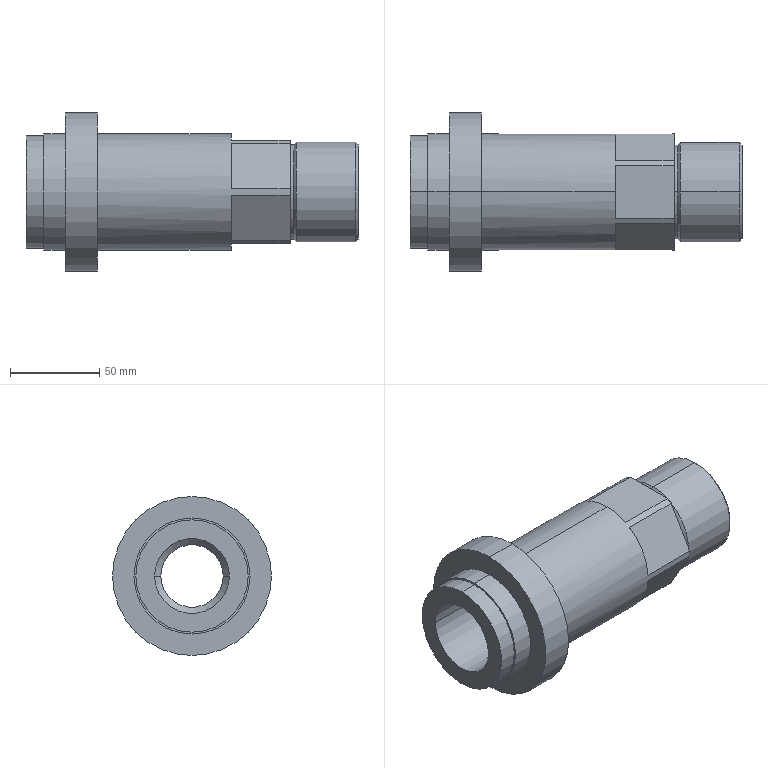Part | SolidWorks | features Chamfer 2, CirPattern 1, ICE 1, RevCut 1, Revolution 1 | 1 solid | 42 faces | box 186 x 89 x 89 mm | volume 390836 mm3 | plane 18 | cylinder 16 | cone 8 | commonest cylinder face diameters 65 x4 35 x2 42 x2 53 x2 56 x2 63 x2
STEP:
#1=CARTESIAN_POINT('',(-3.5,-17.5,0.));
#2=VERTEX_POINT('',#1);
#3=CARTESIAN_POINT('',(-3.5,17.5,0.));
#4=VERTEX_POINT('',#3);
#5=CARTESIAN_POINT('',(-3.5,0.,0.));
#6=DIRECTION('',(1.,0.,0.));
#7=DIRECTION('',(0.,1.,0.));
#8=AXIS2_PLACEMENT_3D('',#5,#6,#7);
#9=CIRCLE('',#8,17.5);
#10=EDGE_CURVE('',#2,#4,#9,.T.);
#11=ORIENTED_EDGE('',*,*,#10,.F.);
#12=CARTESIAN_POINT('',(0.,-21.,0.));
#13=VERTEX_POINT('',#12);
#14=CARTESIAN_POINT('',(-3.5,-17.5,0.));
#15=DIRECTION('',(0.7071,-0.7071,0.));
#16=VECTOR('',#15,1000.);
#17=LINE('',#14,#16);
#18=EDGE_CURVE('',#2,#13,#17,.T.);
#19=ORIENTED_EDGE('',*,*,#18,.T.);
#20=CARTESIAN_POINT('',(0.,21.,0.));
#21=VERTEX_POINT('',#20);
#22=CARTESIAN_POINT('',(0.,0.,0.));
#23=DIRECTION('',(-1.,0.,0.));
#24=DIRECTION('',(0.,0.,-1.));
#25=AXIS2_PLACEMENT_3D('',#22,#23,#24);
#26=CIRCLE('',#25,21.);
#27=EDGE_CURVE('',#21,#13,#26,.T.);
#28=ORIENTED_EDGE('',*,*,#27,.F.);
#29=CARTESIAN_POINT('',(-3.5,17.5,0.));
#30=DIRECTION('',(0.7071,0.7071,0.));
#31=VECTOR('',#30,1000.);
#32=LINE('',#29,#31);
#33=EDGE_CURVE('',#4,#21,#32,.T.);
#34=ORIENTED_EDGE('',*,*,#33,.F.);
#35=EDGE_LOOP('',(#11,#19,#28,#34));
#36=FACE_OUTER_BOUND('',#35,.T.);
#37=CARTESIAN_POINT('',(-3.5,0.,0.));
#38=DIRECTION('',(1.,0.,0.));
#39=DIRECTION('',(0.,1.,0.));
#40=AXIS2_PLACEMENT_3D('',#37,#38,#39);
#41=CONICAL_SURFACE('',#40,17.5,0.7854);
#42=ADVANCED_FACE('',(#36),#41,.F.);
#43=CARTESIAN_POINT('',(-186.,-21.,0.));
#44=VERTEX_POINT('',#43);
#45=CARTESIAN_POINT('',(-186.,21.,0.));
#46=VERTEX_POINT('',#45);
#47=CARTESIAN_POINT('',(-186.,0.,0.));
#48=DIRECTION('',(1.,0.,0.));
#49=DIRECTION('',(0.,1.,0.));
#50=AXIS2_PLACEMENT_3D('',#47,#48,#49);
#51=CIRCLE('',#50,21.);
#52=EDGE_CURVE('',#44,#46,#51,.T.);
#53=ORIENTED_EDGE('',*,*,#52,.F.);
#54=CARTESIAN_POINT('',(-70.,-21.,0.));
#55=VERTEX_POINT('',#54);
#56=CARTESIAN_POINT('',(0.,-21.,0.));
#57=DIRECTION('',(1.,0.,0.));
#58=VECTOR('',#57,1000.);
#59=LINE('',#56,#58);
#60=EDGE_CURVE('',#44,#55,#59,.T.);
#61=ORIENTED_EDGE('',*,*,#60,.T.);
#62=CARTESIAN_POINT('',(-70.,21.,0.));
#63=VERTEX_POINT('',#62);
#64=CARTESIAN_POINT('',(-70.,0.,0.));
#65=DIRECTION('',(1.,0.,0.));
#66=DIRECTION('',(0.,1.,0.));
#67=AXIS2_PLACEMENT_3D('',#64,#65,#66);
#68=CIRCLE('',#67,21.);
#69=EDGE_CURVE('',#55,#63,#68,.T.);
#70=ORIENTED_EDGE('',*,*,#69,.T.);
#71=CARTESIAN_POINT('',(0.,21.,0.));
#72=DIRECTION('',(1.,0.,0.));
#73=VECTOR('',#72,1000.);
#74=LINE('',#71,#73);
#75=EDGE_CURVE('',#46,#63,#74,.T.);
#76=ORIENTED_EDGE('',*,*,#75,.F.);
#77=EDGE_LOOP('',(#53,#61,#70,#76));
#78=FACE_OUTER_BOUND('',#77,.T.);
#79=CARTESIAN_POINT('',(0.,0.,0.));
#80=DIRECTION('',(1.,0.,0.));
#81=DIRECTION('',(0.,1.,0.));
#82=AXIS2_PLACEMENT_3D('',#79,#80,#81);
#83=CYLINDRICAL_SURFACE('',#82,21.);
#84=ADVANCED_FACE('',(#78),#83,.F.);
#85=CARTESIAN_POINT('',(-66.5,-17.5,0.));
#86=VERTEX_POINT('',#85);
#87=CARTESIAN_POINT('',(-66.5,17.5,0.));
#88=VERTEX_POINT('',#87);
#89=CARTESIAN_POINT('',(-66.5,0.,0.));
#90=DIRECTION('',(1.,0.,0.));
#91=DIRECTION('',(0.,1.,0.));
#92=AXIS2_PLACEMENT_3D('',#89,#90,#91);
#93=CIRCLE('',#92,17.5);
#94=EDGE_CURVE('',#86,#88,#93,.T.);
#95=ORIENTED_EDGE('',*,*,#94,.T.);
#96=CARTESIAN_POINT('',(-66.5,17.5,0.));
#97=DIRECTION('',(-0.7071,0.7071,0.));
#98=VECTOR('',#97,1000.);
#99=LINE('',#96,#98);
#100=EDGE_CURVE('',#88,#63,#99,.T.);
#101=ORIENTED_EDGE('',*,*,#100,.T.);
#102=ORIENTED_EDGE('',*,*,#69,.F.);
#103=CARTESIAN_POINT('',(-66.5,-17.5,0.));
#104=DIRECTION('',(-0.7071,-0.7071,0.));
#105=VECTOR('',#104,1000.);
#106=LINE('',#103,#105);
#107=EDGE_CURVE('',#86,#55,#106,.T.);
#108=ORIENTED_EDGE('',*,*,#107,.F.);
#109=EDGE_LOOP('',(#95,#101,#102,#108));
#110=FACE_OUTER_BOUND('',#109,.T.);
#111=CARTESIAN_POINT('',(-66.5,0.,0.));
#112=DIRECTION('',(-1.,0.,0.));
#113=DIRECTION('',(0.,-1.,0.));
#114=AXIS2_PLACEMENT_3D('',#111,#112,#113);
#115=CONICAL_SURFACE('',#114,17.5,0.7854);
#116=ADVANCED_FACE('',(#110),#115,.F.);
#117=ORIENTED_EDGE('',*,*,#94,.F.);
#118=CARTESIAN_POINT('',(0.,-17.5,0.));
#119=DIRECTION('',(1.,0.,0.));
#120=VECTOR('',#119,1000.);
#121=LINE('',#118,#120);
#122=EDGE_CURVE('',#86,#2,#121,.T.);
#123=ORIENTED_EDGE('',*,*,#122,.T.);
#124=ORIENTED_EDGE('',*,*,#10,.T.);
#125=CARTESIAN_POINT('',(0.,17.5,0.));
#126=DIRECTION('',(1.,0.,0.));
#127=VECTOR('',#126,1000.);
#128=LINE('',#125,#127);
#129=EDGE_CURVE('',#88,#4,#128,.T.);
#130=ORIENTED_EDGE('',*,*,#129,.F.);
#131=EDGE_LOOP('',(#117,#123,#124,#130));
#132=FACE_OUTER_BOUND('',#131,.T.);
#133=CARTESIAN_POINT('',(0.,0.,0.));
#134=DIRECTION('',(1.,0.,0.));
#135=DIRECTION('',(0.,1.,0.));
#136=AXIS2_PLACEMENT_3D('',#133,#134,#135);
#137=CYLINDRICAL_SURFACE('',#136,17.5);
#138=ADVANCED_FACE('',(#132),#137,.F.);
#139=CARTESIAN_POINT('',(0.,0.,-26.5));
#140=VERTEX_POINT('',#139);
#141=CARTESIAN_POINT('',(0.,0.,26.5));
#142=VERTEX_POINT('',#141);
#143=CARTESIAN_POINT('',(0.,0.,0.));
#144=DIRECTION('',(1.,0.,0.));
#145=DIRECTION('',(0.,0.,-1.));
#146=AXIS2_PLACEMENT_3D('',#143,#144,#145);
#147=CIRCLE('',#146,26.5);
#148=EDGE_CURVE('',#140,#142,#147,.T.);
#149=ORIENTED_EDGE('',*,*,#148,.F.);
#150=CARTESIAN_POINT('',(-1.5,0.,-28.));
#151=VERTEX_POINT('',#150);
#152=CARTESIAN_POINT('',(0.,0.,-26.5));
#153=DIRECTION('',(-0.7071,0.,-0.7071));
#154=VECTOR('',#153,1000.);
#155=LINE('',#152,#154);
#156=EDGE_CURVE('',#140,#151,#155,.T.);
#157=ORIENTED_EDGE('',*,*,#156,.T.);
#158=CARTESIAN_POINT('',(-1.5,0.,28.));
#159=VERTEX_POINT('',#158);
#160=CARTESIAN_POINT('',(-1.5,0.,0.));
#161=DIRECTION('',(-1.,0.,0.));
#162=DIRECTION('',(0.,0.,-1.));
#163=AXIS2_PLACEMENT_3D('',#160,#161,#162);
#164=CIRCLE('',#163,28.);
#165=EDGE_CURVE('',#159,#151,#164,.T.);
#166=ORIENTED_EDGE('',*,*,#165,.F.);
#167=CARTESIAN_POINT('',(0.,0.,26.5));
#168=DIRECTION('',(-0.7071,0.,0.7071));
#169=VECTOR('',#168,1000.);
#170=LINE('',#167,#169);
#171=EDGE_CURVE('',#142,#159,#170,.T.);
#172=ORIENTED_EDGE('',*,*,#171,.F.);
#173=EDGE_LOOP('',(#149,#157,#166,#172));
#174=FACE_OUTER_BOUND('',#173,.T.);
#175=CARTESIAN_POINT('',(0.,0.,0.));
#176=DIRECTION('',(-1.,0.,0.));
#177=DIRECTION('',(0.,0.,1.));
#178=AXIS2_PLACEMENT_3D('',#175,#176,#177);
#179=CONICAL_SURFACE('',#178,26.5,0.7854);
#180=ADVANCED_FACE('',(#174),#179,.T.);
#181=CARTESIAN_POINT('',(-36.,0.,-26.5));
#182=VERTEX_POINT('',#181);
#183=CARTESIAN_POINT('',(-36.,0.,26.5));
#184=VERTEX_POINT('',#183);
#185=CARTESIAN_POINT('',(-36.,0.,0.));
#186=DIRECTION('',(1.,0.,0.));
#187=DIRECTION('',(0.,0.,-1.));
#188=AXIS2_PLACEMENT_3D('',#185,#186,#187);
#189=CIRCLE('',#188,26.5);
#190=EDGE_CURVE('',#182,#184,#189,.T.);
#191=ORIENTED_EDGE('',*,*,#190,.T.);
#192=CARTESIAN_POINT('',(-34.5,0.,28.));
#193=VERTEX_POINT('',#192);
#194=CARTESIAN_POINT('',(-36.,0.,26.5));
#195=DIRECTION('',(0.7071,0.,0.7071));
#196=VECTOR('',#195,1000.);
#197=LINE('',#194,#196);
#198=EDGE_CURVE('',#184,#193,#197,.T.);
#199=ORIENTED_EDGE('',*,*,#198,.T.);
#200=CARTESIAN_POINT('',(-34.5,0.,-28.));
#201=VERTEX_POINT('',#200);
#202=CARTESIAN_POINT('',(-34.5,0.,0.));
#203=DIRECTION('',(1.,0.,0.));
#204=DIRECTION('',(0.,0.,-1.));
#205=AXIS2_PLACEMENT_3D('',#202,#203,#204);
#206=CIRCLE('',#205,28.);
#207=EDGE_CURVE('',#201,#193,#206,.T.);
#208=ORIENTED_EDGE('',*,*,#207,.F.);
#209=CARTESIAN_POINT('',(-36.,0.,-26.5));
#210=DIRECTION('',(0.7071,0.,-0.7071));
#211=VECTOR('',#210,1000.);
#212=LINE('',#209,#211);
#213=EDGE_CURVE('',#182,#201,#212,.T.);
#214=ORIENTED_EDGE('',*,*,#213,.F.);
#215=EDGE_LOOP('',(#191,#199,#208,#214));
#216=FACE_OUTER_BOUND('',#215,.T.);
#217=CARTESIAN_POINT('',(-36.,0.,0.));
#218=DIRECTION('',(1.,0.,0.));
#219=DIRECTION('',(0.,0.,-1.));
#220=AXIS2_PLACEMENT_3D('',#217,#218,#219);
#221=CONICAL_SURFACE('',#220,26.5,0.7854);
#222=ADVANCED_FACE('',(#216),#221,.T.);
#223=ORIENTED_EDGE('',*,*,#207,.T.);
#224=CARTESIAN_POINT('',(0.,0.,28.));
#225=DIRECTION('',(1.,0.,0.));
#226=VECTOR('',#225,1000.);
#227=LINE('',#224,#226);
#228=EDGE_CURVE('',#193,#159,#227,.T.);
#229=ORIENTED_EDGE('',*,*,#228,.T.);
#230=ORIENTED_EDGE('',*,*,#165,.T.);
#231=CARTESIAN_POINT('',(0.,0.,-28.));
#232=DIRECTION('',(1.,0.,0.));
#233=VECTOR('',#232,1000.);
#234=LINE('',#231,#233);
#235=EDGE_CURVE('',#201,#151,#234,.T.);
#236=ORIENTED_EDGE('',*,*,#235,.F.);
#237=EDGE_LOOP('',(#223,#229,#230,#236));
#238=FACE_OUTER_BOUND('',#237,.T.);
#239=CARTESIAN_POINT('',(0.,0.,0.));
#240=DIRECTION('',(1.,0.,0.));
#241=DIRECTION('',(0.,0.,-1.));
#242=AXIS2_PLACEMENT_3D('',#239,#240,#241);
#243=CYLINDRICAL_SURFACE('',#242,28.);
#244=ADVANCED_FACE('',(#238),#243,.T.);
#245=CARTESIAN_POINT('',(-186.,0.,-31.5));
#246=VERTEX_POINT('',#245);
#247=CARTESIAN_POINT('',(-186.,0.,31.5));
#248=VERTEX_POINT('',#247);
#249=CARTESIAN_POINT('',(-186.,0.,0.));
#250=DIRECTION('',(1.,0.,0.));
#251=DIRECTION('',(0.,0.,-1.));
#252=AXIS2_PLACEMENT_3D('',#249,#250,#251);
#253=CIRCLE('',#252,31.5);
#254=EDGE_CURVE('',#246,#248,#253,.T.);
#255=ORIENTED_EDGE('',*,*,#254,.T.);
#256=CARTESIAN_POINT('',(-176.,0.,31.5));
#257=VERTEX_POINT('',#256);
#258=CARTESIAN_POINT('',(0.,0.,31.5));
#259=DIRECTION('',(1.,0.,0.));
#260=VECTOR('',#259,1000.);
#261=LINE('',#258,#260);
#262=EDGE_CURVE('',#248,#257,#261,.T.);
#263=ORIENTED_EDGE('',*,*,#262,.T.);
#264=CARTESIAN_POINT('',(-176.,0.,-31.5));
#265=VERTEX_POINT('',#264);
#266=CARTESIAN_POINT('',(-176.,0.,0.));
#267=DIRECTION('',(1.,0.,0.));
#268=DIRECTION('',(0.,0.,-1.));
#269=AXIS2_PLACEMENT_3D('',#266,#267,#268);
#270=CIRCLE('',#269,31.5);
#271=EDGE_CURVE('',#265,#257,#270,.T.);
#272=ORIENTED_EDGE('',*,*,#271,.F.);
#273=CARTESIAN_POINT('',(0.,0.,-31.5));
#274=DIRECTION('',(1.,0.,0.));
#275=VECTOR('',#274,1000.);
#276=LINE('',#273,#275);
#277=EDGE_CURVE('',#246,#265,#276,.T.);
#278=ORIENTED_EDGE('',*,*,#277,.F.);
#279=EDGE_LOOP('',(#255,#263,#272,#278));
#280=FACE_OUTER_BOUND('',#279,.T.);
#281=CARTESIAN_POINT('',(0.,0.,0.));
#282=DIRECTION('',(1.,0.,0.));
#283=DIRECTION('',(0.,0.,-1.));
#284=AXIS2_PLACEMENT_3D('',#281,#282,#283);
#285=CYLINDRICAL_SURFACE('',#284,31.5);
#286=ADVANCED_FACE('',(#280),#285,.T.);
#287=CARTESIAN_POINT('',(-176.,0.,-32.5));
#288=VERTEX_POINT('',#287);
#289=CARTESIAN_POINT('',(-176.,0.,32.5));
#290=VERTEX_POINT('',#289);
#291=CARTESIAN_POINT('',(-176.,0.,0.));
#292=DIRECTION('',(1.,0.,0.));
#293=DIRECTION('',(0.,0.,-1.));
#294=AXIS2_PLACEMENT_3D('',#291,#292,#293);
#295=CIRCLE('',#294,32.5);
#296=EDGE_CURVE('',#288,#290,#295,.T.);
#297=ORIENTED_EDGE('',*,*,#296,.T.);
#298=CARTESIAN_POINT('',(-164.,0.,32.5));
#299=VERTEX_POINT('',#298);
#300=CARTESIAN_POINT('',(0.,0.,32.5));
#301=DIRECTION('',(1.,0.,0.));
#302=VECTOR('',#301,1000.);
#303=LINE('',#300,#302);
#304=EDGE_CURVE('',#290,#299,#303,.T.);
#305=ORIENTED_EDGE('',*,*,#304,.T.);
#306=CARTESIAN_POINT('',(-164.,0.,-32.5));
#307=VERTEX_POINT('',#306);
#308=CARTESIAN_POINT('',(-164.,0.,0.));
#309=DIRECTION('',(1.,0.,0.));
#310=DIRECTION('',(0.,0.,-1.));
#311=AXIS2_PLACEMENT_3D('',#308,#309,#310);
#312=CIRCLE('',#311,32.5);
#313=EDGE_CURVE('',#307,#299,#312,.T.);
#314=ORIENTED_EDGE('',*,*,#313,.F.);
#315=CARTESIAN_POINT('',(0.,0.,-32.5));
#316=DIRECTION('',(1.,0.,0.));
#317=VECTOR('',#316,1000.);
#318=LINE('',#315,#317);
#319=EDGE_CURVE('',#288,#307,#318,.T.);
#320=ORIENTED_EDGE('',*,*,#319,.F.);
#321=EDGE_LOOP('',(#297,#305,#314,#320));
#322=FACE_OUTER_BOUND('',#321,.T.);
#323=CARTESIAN_POINT('',(0.,0.,0.));
#324=DIRECTION('',(1.,0.,0.));
#325=DIRECTION('',(0.,0.,-1.));
#326=AXIS2_PLACEMENT_3D('',#323,#324,#325);
#327=CYLINDRICAL_SURFACE('',#326,32.5);
#328=ADVANCED_FACE('',(#322),#327,.T.);
#329=CARTESIAN_POINT('',(-164.,0.,-44.5));
#330=VERTEX_POINT('',#329);
#331=CARTESIAN_POINT('',(-164.,0.,44.5));
#332=VERTEX_POINT('',#331);
#333=CARTESIAN_POINT('',(-164.,0.,0.));
#334=DIRECTION('',(1.,0.,0.));
#335=DIRECTION('',(0.,0.,-1.));
#336=AXIS2_PLACEMENT_3D('',#333,#334,#335);
#337=CIRCLE('',#336,44.5);
#338=EDGE_CURVE('',#330,#332,#337,.T.);
#339=ORIENTED_EDGE('',*,*,#338,.T.);
#340=CARTESIAN_POINT('',(-146.,0.,44.5));
#341=VERTEX_POINT('',#340);
#342=CARTESIAN_POINT('',(0.,0.,44.5));
#343=DIRECTION('',(1.,0.,0.));
#344=VECTOR('',#343,1000.);
#345=LINE('',#342,#344);
#346=EDGE_CURVE('',#332,#341,#345,.T.);
#347=ORIENTED_EDGE('',*,*,#346,.T.);
#348=CARTESIAN_POINT('',(-146.,0.,-44.5));
#349=VERTEX_POINT('',#348);
#350=CARTESIAN_POINT('',(-146.,0.,0.));
#351=DIRECTION('',(1.,0.,0.));
#352=DIRECTION('',(0.,0.,-1.));
#353=AXIS2_PLACEMENT_3D('',#350,#351,#352);
#354=CIRCLE('',#353,44.5);
#355=EDGE_CURVE('',#349,#341,#354,.T.);
#356=ORIENTED_EDGE('',*,*,#355,.F.);
#357=CARTESIAN_POINT('',(0.,0.,-44.5));
#358=DIRECTION('',(1.,0.,0.));
#359=VECTOR('',#358,1000.);
#360=LINE('',#357,#359);
#361=EDGE_CURVE('',#330,#349,#360,.T.);
#362=ORIENTED_EDGE('',*,*,#361,.F.);
#363=EDGE_LOOP('',(#339,#347,#356,#362));
#364=FACE_OUTER_BOUND('',#363,.T.);
#365=CARTESIAN_POINT('',(0.,0.,0.));
#366=DIRECTION('',(1.,0.,0.));
#367=DIRECTION('',(0.,0.,-1.));
#368=AXIS2_PLACEMENT_3D('',#365,#366,#367);
#369=CYLINDRICAL_SURFACE('',#368,44.5);
#370=ADVANCED_FACE('',(#364),#369,.T.);
#371=CARTESIAN_POINT('',(-146.,0.,-32.5));
#372=VERTEX_POINT('',#371);
#373=CARTESIAN_POINT('',(-146.,0.,32.5));
#374=VERTEX_POINT('',#373);
#375=CARTESIAN_POINT('',(-146.,0.,0.));
#376=DIRECTION('',(1.,0.,0.));
#377=DIRECTION('',(0.,0.,-1.));
#378=AXIS2_PLACEMENT_3D('',#375,#376,#377);
#379=CIRCLE('',#378,32.5);
#380=EDGE_CURVE('',#372,#374,#379,.T.);
#381=ORIENTED_EDGE('',*,*,#380,.T.);
#382=CARTESIAN_POINT('',(-71.,0.,32.5));
#383=VERTEX_POINT('',#382);
#384=CARTESIAN_POINT('',(0.,0.,32.5));
#385=DIRECTION('',(1.,0.,0.));
#386=VECTOR('',#385,1000.);
#387=LINE('',#384,#386);
#388=EDGE_CURVE('',#374,#383,#387,.T.);
#389=ORIENTED_EDGE('',*,*,#388,.T.);
#390=CARTESIAN_POINT('',(-71.,14.671,29.));
#391=VERTEX_POINT('',#390);
#392=CARTESIAN_POINT('',(-71.,0.,0.));
#393=DIRECTION('',(1.,0.,0.));
#394=DIRECTION('',(0.,0.,-1.));
#395=AXIS2_PLACEMENT_3D('',#392,#393,#394);
#396=CIRCLE('',#395,32.5);
#397=EDGE_CURVE('',#391,#383,#396,.T.);
#398=ORIENTED_EDGE('',*,*,#397,.F.);
#399=CARTESIAN_POINT('',(-38.,14.671,29.));
#400=VERTEX_POINT('',#399);
#401=CARTESIAN_POINT('',(-71.,14.671,29.));
#402=DIRECTION('',(1.,0.,0.));
#403=VECTOR('',#402,1000.);
#404=LINE('',#401,#403);
#405=EDGE_CURVE('',#391,#400,#404,.T.);
#406=ORIENTED_EDGE('',*,*,#405,.T.);
#407=CARTESIAN_POINT('',(-38.,17.779,27.206));
#408=VERTEX_POINT('',#407);
#409=CARTESIAN_POINT('',(-38.,0.,0.));
#410=DIRECTION('',(1.,0.,0.));
#411=DIRECTION('',(0.,0.,-1.));
#412=AXIS2_PLACEMENT_3D('',#409,#410,#411);
#413=CIRCLE('',#412,32.5);
#414=EDGE_CURVE('',#408,#400,#413,.T.);
#415=ORIENTED_EDGE('',*,*,#414,.F.);
#416=CARTESIAN_POINT('',(-71.,17.779,27.206));
#417=VERTEX_POINT('',#416);
#418=CARTESIAN_POINT('',(-71.,17.779,27.206));
#419=DIRECTION('',(1.,0.,0.));
#420=VECTOR('',#419,1000.);
#421=LINE('',#418,#420);
#422=EDGE_CURVE('',#417,#408,#421,.T.);
#423=ORIENTED_EDGE('',*,*,#422,.F.);
#424=CARTESIAN_POINT('',(-71.,32.45,1.794));
#425=VERTEX_POINT('',#424);
#426=CARTESIAN_POINT('',(-71.,0.,0.));
#427=DIRECTION('',(1.,0.,0.));
#428=DIRECTION('',(0.,0.,-1.));
#429=AXIS2_PLACEMENT_3D('',#426,#427,#428);
#430=CIRCLE('',#429,32.5);
#431=EDGE_CURVE('',#425,#417,#430,.T.);
#432=ORIENTED_EDGE('',*,*,#431,.F.);
#433=CARTESIAN_POINT('',(-38.,32.45,1.794));
#434=VERTEX_POINT('',#433);
#435=CARTESIAN_POINT('',(-71.,32.45,1.794));
#436=DIRECTION('',(1.,0.,0.));
#437=VECTOR('',#436,1000.);
#438=LINE('',#435,#437);
#439=EDGE_CURVE('',#425,#434,#438,.T.);
#440=ORIENTED_EDGE('',*,*,#439,.T.);
#441=CARTESIAN_POINT('',(-38.,32.45,-1.794));
#442=VERTEX_POINT('',#441);
#443=CARTESIAN_POINT('',(-38.,0.,0.));
#444=DIRECTION('',(1.,0.,0.));
#445=DIRECTION('',(0.,0.,-1.));
#446=AXIS2_PLACEMENT_3D('',#443,#444,#445);
#447=CIRCLE('',#446,32.5);
#448=EDGE_CURVE('',#442,#434,#447,.T.);
#449=ORIENTED_EDGE('',*,*,#448,.F.);
#450=CARTESIAN_POINT('',(-71.,32.45,-1.794));
#451=VERTEX_POINT('',#450);
#452=CARTESIAN_POINT('',(-71.,32.45,-1.794));
#453=DIRECTION('',(1.,0.,0.));
#454=VECTOR('',#453,1000.);
#455=LINE('',#452,#454);
#456=EDGE_CURVE('',#451,#442,#455,.T.);
#457=ORIENTED_EDGE('',*,*,#456,.F.);
#458=CARTESIAN_POINT('',(-71.,17.779,-27.206));
#459=VERTEX_POINT('',#458);
#460=CARTESIAN_POINT('',(-71.,0.,0.));
#461=DIRECTION('',(1.,0.,0.));
#462=DIRECTION('',(0.,0.,-1.));
#463=AXIS2_PLACEMENT_3D('',#460,#461,#462);
#464=CIRCLE('',#463,32.5);
#465=EDGE_CURVE('',#459,#451,#464,.T.);
#466=ORIENTED_EDGE('',*,*,#465,.F.);
#467=CARTESIAN_POINT('',(-38.,17.779,-27.206));
#468=VERTEX_POINT('',#467);
#469=CARTESIAN_POINT('',(-71.,17.779,-27.206));
#470=DIRECTION('',(1.,0.,0.));
#471=VECTOR('',#470,1000.);
#472=LINE('',#469,#471);
#473=EDGE_CURVE('',#459,#468,#472,.T.);
#474=ORIENTED_EDGE('',*,*,#473,.T.);
#475=CARTESIAN_POINT('',(-38.,14.671,-29.));
#476=VERTEX_POINT('',#475);
#477=CARTESIAN_POINT('',(-38.,0.,0.));
#478=DIRECTION('',(1.,0.,0.));
#479=DIRECTION('',(0.,0.,-1.));
#480=AXIS2_PLACEMENT_3D('',#477,#478,#479);
#481=CIRCLE('',#480,32.5);
#482=EDGE_CURVE('',#476,#468,#481,.T.);
#483=ORIENTED_EDGE('',*,*,#482,.F.);
#484=CARTESIAN_POINT('',(-71.,14.671,-29.));
#485=VERTEX_POINT('',#484);
#486=CARTESIAN_POINT('',(-71.,14.671,-29.));
#487=DIRECTION('',(1.,0.,0.));
#488=VECTOR('',#487,1000.);
#489=LINE('',#486,#488);
#490=EDGE_CURVE('',#485,#476,#489,.T.);
#491=ORIENTED_EDGE('',*,*,#490,.F.);
#492=CARTESIAN_POINT('',(-71.,0.,-32.5));
#493=VERTEX_POINT('',#492);
#494=CARTESIAN_POINT('',(-71.,0.,0.));
#495=DIRECTION('',(1.,0.,0.));
#496=DIRECTION('',(0.,0.,-1.));
#497=AXIS2_PLACEMENT_3D('',#494,#495,#496);
#498=CIRCLE('',#497,32.5);
#499=EDGE_CURVE('',#493,#485,#498,.T.);
#500=ORIENTED_EDGE('',*,*,#499,.F.);
#501=CARTESIAN_POINT('',(0.,0.,-32.5));
#502=DIRECTION('',(1.,0.,0.));
#503=VECTOR('',#502,1000.);
#504=LINE('',#501,#503);
#505=EDGE_CURVE('',#372,#493,#504,.T.);
#506=ORIENTED_EDGE('',*,*,#505,.F.);
#507=EDGE_LOOP('',(#381,#389,#398,#406,#415,#423,#432,#440,#449,#457,#466,#474,#483,#491,#500,#506));
#508=FACE_OUTER_BOUND('',#507,.T.);
#509=CARTESIAN_POINT('',(0.,0.,0.));
#510=DIRECTION('',(1.,0.,0.));
#511=DIRECTION('',(0.,0.,-1.));
#512=AXIS2_PLACEMENT_3D('',#509,#510,#511);
#513=CYLINDRICAL_SURFACE('',#512,32.5);
#514=ADVANCED_FACE('',(#508),#513,.T.);
#515=CARTESIAN_POINT('',(-38.,0.,-26.5));
#516=VERTEX_POINT('',#515);
#517=CARTESIAN_POINT('',(-38.,0.,26.5));
#518=VERTEX_POINT('',#517);
#519=CARTESIAN_POINT('',(-38.,0.,0.));
#520=DIRECTION('',(1.,0.,0.));
#521=DIRECTION('',(0.,0.,-1.));
#522=AXIS2_PLACEMENT_3D('',#519,#520,#521);
#523=CIRCLE('',#522,26.5);
#524=EDGE_CURVE('',#516,#518,#523,.T.);
#525=ORIENTED_EDGE('',*,*,#524,.T.);
#526=CARTESIAN_POINT('',(0.,0.,26.5));
#527=DIRECTION('',(1.,0.,0.));
#528=VECTOR('',#527,1000.);
#529=LINE('',#526,#528);
#530=EDGE_CURVE('',#518,#184,#529,.T.);
#531=ORIENTED_EDGE('',*,*,#530,.T.);
#532=ORIENTED_EDGE('',*,*,#190,.F.);
#533=CARTESIAN_POINT('',(0.,0.,-26.5));
#534=DIRECTION('',(1.,0.,0.));
#535=VECTOR('',#534,1000.);
#536=LINE('',#533,#535);
#537=EDGE_CURVE('',#516,#182,#536,.T.);
#538=ORIENTED_EDGE('',*,*,#537,.F.);
#539=EDGE_LOOP('',(#525,#531,#532,#538));
#540=FACE_OUTER_BOUND('',#539,.T.);
#541=CARTESIAN_POINT('',(0.,0.,0.));
#542=DIRECTION('',(1.,0.,0.));
#543=DIRECTION('',(0.,0.,-1.));
#544=AXIS2_PLACEMENT_3D('',#541,#542,#543);
#545=CYLINDRICAL_SURFACE('',#544,26.5);
#546=ADVANCED_FACE('',(#540),#545,.T.);
#547=ORIENTED_EDGE('',*,*,#530,.F.);
#548=CARTESIAN_POINT('',(-38.,0.,0.));
#549=DIRECTION('',(1.,0.,0.));
#550=DIRECTION('',(0.,0.,-1.));
#551=AXIS2_PLACEMENT_3D('',#548,#549,#550);
#552=CIRCLE('',#551,26.5);
#553=EDGE_CURVE('',#518,#516,#552,.T.);
#554=ORIENTED_EDGE('',*,*,#553,.T.);
#555=ORIENTED_EDGE('',*,*,#537,.T.);
#556=CARTESIAN_POINT('',(-36.,0.,0.));
#557=DIRECTION('',(1.,0.,0.));
#558=DIRECTION('',(0.,0.,-1.));
#559=AXIS2_PLACEMENT_3D('',#556,#557,#558);
#560=CIRCLE('',#559,26.5);
#561=EDGE_CURVE('',#184,#182,#560,.T.);
#562=ORIENTED_EDGE('',*,*,#561,.F.);
#563=EDGE_LOOP('',(#547,#554,#555,#562));
#564=FACE_OUTER_BOUND('',#563,.T.);
#565=CARTESIAN_POINT('',(0.,0.,0.));
#566=DIRECTION('',(1.,0.,0.));
#567=DIRECTION('',(0.,0.,-1.));
#568=AXIS2_PLACEMENT_3D('',#565,#566,#567);
#569=CYLINDRICAL_SURFACE('',#568,26.5);
#570=ADVANCED_FACE('',(#564),#569,.T.);
#571=CARTESIAN_POINT('',(-38.,-14.671,-29.));
#572=VERTEX_POINT('',#571);
#573=CARTESIAN_POINT('',(-38.,0.,-29.));
#574=DIRECTION('',(0.,-1.,0.));
#575=VECTOR('',#574,1000.);
#576=LINE('',#573,#575);
#577=EDGE_CURVE('',#476,#572,#576,.T.);
#578=ORIENTED_EDGE('',*,*,#577,.F.);
#579=ORIENTED_EDGE('',*,*,#482,.T.);
#580=CARTESIAN_POINT('',(-38.,25.115,-14.5));
#581=DIRECTION('',(0.,-0.5,-0.866));
#582=VECTOR('',#581,1000.);
#583=LINE('',#580,#582);
#584=EDGE_CURVE('',#442,#468,#583,.T.);
#585=ORIENTED_EDGE('',*,*,#584,.F.);
#586=ORIENTED_EDGE('',*,*,#448,.T.);
#587=CARTESIAN_POINT('',(-38.,25.115,14.5));
#588=DIRECTION('',(0.,0.5,-0.866));
#589=VECTOR('',#588,1000.);
#590=LINE('',#587,#589);
#591=EDGE_CURVE('',#408,#434,#590,.T.);
#592=ORIENTED_EDGE('',*,*,#591,.F.);
#593=ORIENTED_EDGE('',*,*,#414,.T.);
#594=CARTESIAN_POINT('',(-38.,-14.671,29.));
#595=VERTEX_POINT('',#594);
#596=CARTESIAN_POINT('',(-38.,0.,29.));
#597=DIRECTION('',(0.,1.,0.));
#598=VECTOR('',#597,1000.);
#599=LINE('',#596,#598);
#600=EDGE_CURVE('',#595,#400,#599,.T.);
#601=ORIENTED_EDGE('',*,*,#600,.F.);
#602=CARTESIAN_POINT('',(-38.,-17.779,27.206));
#603=VERTEX_POINT('',#602);
#604=CARTESIAN_POINT('',(-38.,0.,0.));
#605=DIRECTION('',(1.,0.,0.));
#606=DIRECTION('',(0.,0.,-1.));
#607=AXIS2_PLACEMENT_3D('',#604,#605,#606);
#608=CIRCLE('',#607,32.5);
#609=EDGE_CURVE('',#595,#603,#608,.T.);
#610=ORIENTED_EDGE('',*,*,#609,.T.);
#611=CARTESIAN_POINT('',(-38.,-32.45,1.794));
#612=VERTEX_POINT('',#611);
#613=CARTESIAN_POINT('',(-38.,-25.115,14.5));
#614=DIRECTION('',(0.,0.5,0.866));
#615=VECTOR('',#614,1000.);
#616=LINE('',#613,#615);
#617=EDGE_CURVE('',#612,#603,#616,.T.);
#618=ORIENTED_EDGE('',*,*,#617,.F.);
#619=CARTESIAN_POINT('',(-38.,-32.45,-1.794));
#620=VERTEX_POINT('',#619);
#621=CARTESIAN_POINT('',(-38.,0.,0.));
#622=DIRECTION('',(1.,0.,0.));
#623=DIRECTION('',(0.,0.,-1.));
#624=AXIS2_PLACEMENT_3D('',#621,#622,#623);
#625=CIRCLE('',#624,32.5);
#626=EDGE_CURVE('',#612,#620,#625,.T.);
#627=ORIENTED_EDGE('',*,*,#626,.T.);
#628=CARTESIAN_POINT('',(-38.,-17.779,-27.206));
#629=VERTEX_POINT('',#628);
#630=CARTESIAN_POINT('',(-38.,-25.115,-14.5));
#631=DIRECTION('',(0.,-0.5,0.866));
#632=VECTOR('',#631,1000.);
#633=LINE('',#630,#632);
#634=EDGE_CURVE('',#629,#620,#633,.T.);
#635=ORIENTED_EDGE('',*,*,#634,.F.);
#636=CARTESIAN_POINT('',(-38.,0.,0.));
#637=DIRECTION('',(1.,0.,0.));
#638=DIRECTION('',(0.,0.,-1.));
#639=AXIS2_PLACEMENT_3D('',#636,#637,#638);
#640=CIRCLE('',#639,32.5);
#641=EDGE_CURVE('',#629,#572,#640,.T.);
#642=ORIENTED_EDGE('',*,*,#641,.T.);
#643=EDGE_LOOP('',(#578,#579,#585,#586,#592,#593,#601,#610,#618,#627,#635,#642));
#644=FACE_OUTER_BOUND('',#643,.T.);
#645=ORIENTED_EDGE('',*,*,#524,.F.);
#646=ORIENTED_EDGE('',*,*,#553,.F.);
#647=EDGE_LOOP('',(#645,#646));
#648=FACE_BOUND('',#647,.T.);
#649=CARTESIAN_POINT('',(-38.,0.,0.));
#650=DIRECTION('',(1.,0.,0.));
#651=DIRECTION('',(0.,0.,-1.));
#652=AXIS2_PLACEMENT_3D('',#649,#650,#651);
#653=PLANE('',#652);
#654=ADVANCED_FACE('',(#644,#648),#653,.T.);
#655=ORIENTED_EDGE('',*,*,#388,.F.);
#656=CARTESIAN_POINT('',(-146.,0.,0.));
#657=DIRECTION('',(1.,0.,0.));
#658=DIRECTION('',(0.,0.,-1.));
#659=AXIS2_PLACEMENT_3D('',#656,#657,#658);
#660=CIRCLE('',#659,32.5);
#661=EDGE_CURVE('',#374,#372,#660,.T.);
#662=ORIENTED_EDGE('',*,*,#661,.T.);
#663=ORIENTED_EDGE('',*,*,#505,.T.);
#664=CARTESIAN_POINT('',(-71.,-14.671,-29.));
#665=VERTEX_POINT('',#664);
#666=CARTESIAN_POINT('',(-71.,0.,0.));
#667=DIRECTION('',(1.,0.,0.));
#668=DIRECTION('',(0.,0.,-1.));
#669=AXIS2_PLACEMENT_3D('',#666,#667,#668);
#670=CIRCLE('',#669,32.5);
#671=EDGE_CURVE('',#665,#493,#670,.T.);
#672=ORIENTED_EDGE('',*,*,#671,.F.);
#673=CARTESIAN_POINT('',(-71.,-14.671,-29.));
#674=DIRECTION('',(1.,0.,0.));
#675=VECTOR('',#674,1000.);
#676=LINE('',#673,#675);
#677=EDGE_CURVE('',#665,#572,#676,.T.);
#678=ORIENTED_EDGE('',*,*,#677,.T.);
#679=ORIENTED_EDGE('',*,*,#641,.F.);
#680=CARTESIAN_POINT('',(-71.,-17.779,-27.206));
#681=VERTEX_POINT('',#680);
#682=CARTESIAN_POINT('',(-71.,-17.779,-27.206));
#683=DIRECTION('',(1.,0.,0.));
#684=VECTOR('',#683,1000.);
#685=LINE('',#682,#684);
#686=EDGE_CURVE('',#681,#629,#685,.T.);
#687=ORIENTED_EDGE('',*,*,#686,.F.);
#688=CARTESIAN_POINT('',(-71.,-32.45,-1.794));
#689=VERTEX_POINT('',#688);
#690=CARTESIAN_POINT('',(-71.,0.,0.));
#691=DIRECTION('',(1.,0.,0.));
#692=DIRECTION('',(0.,0.,-1.));
#693=AXIS2_PLACEMENT_3D('',#690,#691,#692);
#694=CIRCLE('',#693,32.5);
#695=EDGE_CURVE('',#689,#681,#694,.T.);
#696=ORIENTED_EDGE('',*,*,#695,.F.);
#697=CARTESIAN_POINT('',(-71.,-32.45,-1.794));
#698=DIRECTION('',(1.,0.,0.));
#699=VECTOR('',#698,1000.);
#700=LINE('',#697,#699);
#701=EDGE_CURVE('',#689,#620,#700,.T.);
#702=ORIENTED_EDGE('',*,*,#701,.T.);
#703=ORIENTED_EDGE('',*,*,#626,.F.);
#704=CARTESIAN_POINT('',(-71.,-32.45,1.794));
#705=VERTEX_POINT('',#704);
#706=CARTESIAN_POINT('',(-71.,-32.45,1.794));
#707=DIRECTION('',(1.,0.,0.));
#708=VECTOR('',#707,1000.);
#709=LINE('',#706,#708);
#710=EDGE_CURVE('',#705,#612,#709,.T.);
#711=ORIENTED_EDGE('',*,*,#710,.F.);
#712=CARTESIAN_POINT('',(-71.,-17.779,27.206));
#713=VERTEX_POINT('',#712);
#714=CARTESIAN_POINT('',(-71.,0.,0.));
#715=DIRECTION('',(1.,0.,0.));
#716=DIRECTION('',(0.,0.,-1.));
#717=AXIS2_PLACEMENT_3D('',#714,#715,#716);
#718=CIRCLE('',#717,32.5);
#719=EDGE_CURVE('',#713,#705,#718,.T.);
#720=ORIENTED_EDGE('',*,*,#719,.F.);
#721=CARTESIAN_POINT('',(-71.,-17.779,27.206));
#722=DIRECTION('',(1.,0.,0.));
#723=VECTOR('',#722,1000.);
#724=LINE('',#721,#723);
#725=EDGE_CURVE('',#713,#603,#724,.T.);
#726=ORIENTED_EDGE('',*,*,#725,.T.);
#727=ORIENTED_EDGE('',*,*,#609,.F.);
#728=CARTESIAN_POINT('',(-71.,-14.671,29.));
#729=VERTEX_POINT('',#728);
#730=CARTESIAN_POINT('',(-71.,-14.671,29.));
#731=DIRECTION('',(1.,0.,0.));
#732=VECTOR('',#731,1000.);
#733=LINE('',#730,#732);
#734=EDGE_CURVE('',#729,#595,#733,.T.);
#735=ORIENTED_EDGE('',*,*,#734,.F.);
#736=CARTESIAN_POINT('',(-71.,0.,0.));
#737=DIRECTION('',(1.,0.,0.));
#738=DIRECTION('',(0.,0.,-1.));
#739=AXIS2_PLACEMENT_3D('',#736,#737,#738);
#740=CIRCLE('',#739,32.5);
#741=EDGE_CURVE('',#383,#729,#740,.T.);
#742=ORIENTED_EDGE('',*,*,#741,.F.);
#743=EDGE_LOOP('',(#655,#662,#663,#672,#678,#679,#687,#696,#702,#703,#711,#720,#726,#727,#735,#742));
#744=FACE_OUTER_BOUND('',#743,.T.);
#745=CARTESIAN_POINT('',(0.,0.,0.));
#746=DIRECTION('',(1.,0.,0.));
#747=DIRECTION('',(0.,0.,-1.));
#748=AXIS2_PLACEMENT_3D('',#745,#746,#747);
#749=CYLINDRICAL_SURFACE('',#748,32.5);
#750=ADVANCED_FACE('',(#744),#749,.T.);
#751=ORIENTED_EDGE('',*,*,#355,.T.);
#752=CARTESIAN_POINT('',(-146.,0.,0.));
#753=DIRECTION('',(1.,0.,0.));
#754=DIRECTION('',(0.,0.,-1.));
#755=AXIS2_PLACEMENT_3D('',#752,#753,#754);
#756=CIRCLE('',#755,44.5);
#757=EDGE_CURVE('',#341,#349,#756,.T.);
#758=ORIENTED_EDGE('',*,*,#757,.T.);
#759=EDGE_LOOP('',(#751,#758));
#760=FACE_OUTER_BOUND('',#759,.T.);
#761=ORIENTED_EDGE('',*,*,#380,.F.);
#762=ORIENTED_EDGE('',*,*,#661,.F.);
#763=EDGE_LOOP('',(#761,#762));
#764=FACE_BOUND('',#763,.T.);
#765=CARTESIAN_POINT('',(-146.,0.,0.));
#766=DIRECTION('',(1.,0.,0.));
#767=DIRECTION('',(0.,0.,-1.));
#768=AXIS2_PLACEMENT_3D('',#765,#766,#767);
#769=PLANE('',#768);
#770=ADVANCED_FACE('',(#760,#764),#769,.T.);
#771=ORIENTED_EDGE('',*,*,#346,.F.);
#772=CARTESIAN_POINT('',(-164.,0.,0.));
#773=DIRECTION('',(1.,0.,0.));
#774=DIRECTION('',(0.,0.,-1.));
#775=AXIS2_PLACEMENT_3D('',#772,#773,#774);
#776=CIRCLE('',#775,44.5);
#777=EDGE_CURVE('',#332,#330,#776,.T.);
#778=ORIENTED_EDGE('',*,*,#777,.T.);
#779=ORIENTED_EDGE('',*,*,#361,.T.);
#780=ORIENTED_EDGE('',*,*,#757,.F.);
#781=EDGE_LOOP('',(#771,#778,#779,#780));
#782=FACE_OUTER_BOUND('',#781,.T.);
#783=CARTESIAN_POINT('',(0.,0.,0.));
#784=DIRECTION('',(1.,0.,0.));
#785=DIRECTION('',(0.,0.,-1.));
#786=AXIS2_PLACEMENT_3D('',#783,#784,#785);
#787=CYLINDRICAL_SURFACE('',#786,44.5);
#788=ADVANCED_FACE('',(#782),#787,.T.);
#789=ORIENTED_EDGE('',*,*,#338,.F.);
#790=ORIENTED_EDGE('',*,*,#777,.F.);
#791=EDGE_LOOP('',(#789,#790));
#792=FACE_OUTER_BOUND('',#791,.T.);
#793=ORIENTED_EDGE('',*,*,#313,.T.);
#794=CARTESIAN_POINT('',(-164.,0.,0.));
#795=DIRECTION('',(1.,0.,0.));
#796=DIRECTION('',(0.,0.,-1.));
#797=AXIS2_PLACEMENT_3D('',#794,#795,#796);
#798=CIRCLE('',#797,32.5);
#799=EDGE_CURVE('',#299,#307,#798,.T.);
#800=ORIENTED_EDGE('',*,*,#799,.T.);
#801=EDGE_LOOP('',(#793,#800));
#802=FACE_BOUND('',#801,.T.);
#803=CARTESIAN_POINT('',(-164.,0.,0.));
#804=DIRECTION('',(1.,0.,0.));
#805=DIRECTION('',(0.,0.,-1.));
#806=AXIS2_PLACEMENT_3D('',#803,#804,#805);
#807=PLANE('',#806);
#808=ADVANCED_FACE('',(#792,#802),#807,.F.);
#809=ORIENTED_EDGE('',*,*,#304,.F.);
#810=CARTESIAN_POINT('',(-176.,0.,0.));
#811=DIRECTION('',(1.,0.,0.));
#812=DIRECTION('',(0.,0.,-1.));
#813=AXIS2_PLACEMENT_3D('',#810,#811,#812);
#814=CIRCLE('',#813,32.5);
#815=EDGE_CURVE('',#290,#288,#814,.T.);
#816=ORIENTED_EDGE('',*,*,#815,.T.);
#817=ORIENTED_EDGE('',*,*,#319,.T.);
#818=ORIENTED_EDGE('',*,*,#799,.F.);
#819=EDGE_LOOP('',(#809,#816,#817,#818));
#820=FACE_OUTER_BOUND('',#819,.T.);
#821=CARTESIAN_POINT('',(0.,0.,0.));
#822=DIRECTION('',(1.,0.,0.));
#823=DIRECTION('',(0.,0.,-1.));
#824=AXIS2_PLACEMENT_3D('',#821,#822,#823);
#825=CYLINDRICAL_SURFACE('',#824,32.5);
#826=ADVANCED_FACE('',(#820),#825,.T.);
#827=ORIENTED_EDGE('',*,*,#296,.F.);
#828=ORIENTED_EDGE('',*,*,#815,.F.);
#829=EDGE_LOOP('',(#827,#828));
#830=FACE_OUTER_BOUND('',#829,.T.);
#831=ORIENTED_EDGE('',*,*,#271,.T.);
#832=CARTESIAN_POINT('',(-176.,0.,0.));
#833=DIRECTION('',(1.,0.,0.));
#834=DIRECTION('',(0.,0.,-1.));
#835=AXIS2_PLACEMENT_3D('',#832,#833,#834);
#836=CIRCLE('',#835,31.5);
#837=EDGE_CURVE('',#257,#265,#836,.T.);
#838=ORIENTED_EDGE('',*,*,#837,.T.);
#839=EDGE_LOOP('',(#831,#838));
#840=FACE_BOUND('',#839,.T.);
#841=CARTESIAN_POINT('',(-176.,0.,0.));
#842=DIRECTION('',(1.,0.,0.));
#843=DIRECTION('',(0.,0.,-1.));
#844=AXIS2_PLACEMENT_3D('',#841,#842,#843);
#845=PLANE('',#844);
#846=ADVANCED_FACE('',(#830,#840),#845,.F.);
#847=ORIENTED_EDGE('',*,*,#262,.F.);
#848=CARTESIAN_POINT('',(-186.,0.,0.));
#849=DIRECTION('',(1.,0.,0.));
#850=DIRECTION('',(0.,0.,-1.));
#851=AXIS2_PLACEMENT_3D('',#848,#849,#850);
#852=CIRCLE('',#851,31.5);
#853=EDGE_CURVE('',#248,#246,#852,.T.);
#854=ORIENTED_EDGE('',*,*,#853,.T.);
#855=ORIENTED_EDGE('',*,*,#277,.T.);
#856=ORIENTED_EDGE('',*,*,#837,.F.);
#857=EDGE_LOOP('',(#847,#854,#855,#856));
#858=FACE_OUTER_BOUND('',#857,.T.);
#859=CARTESIAN_POINT('',(0.,0.,0.));
#860=DIRECTION('',(1.,0.,0.));
#861=DIRECTION('',(0.,0.,-1.));
#862=AXIS2_PLACEMENT_3D('',#859,#860,#861);
#863=CYLINDRICAL_SURFACE('',#862,31.5);
#864=ADVANCED_FACE('',(#858),#863,.T.);
#865=CARTESIAN_POINT('',(-186.,0.,0.));
#866=DIRECTION('',(1.,0.,0.));
#867=DIRECTION('',(0.,1.,0.));
#868=AXIS2_PLACEMENT_3D('',#865,#866,#867);
#869=CIRCLE('',#868,21.);
#870=EDGE_CURVE('',#46,#44,#869,.T.);
#871=ORIENTED_EDGE('',*,*,#870,.T.);
#872=ORIENTED_EDGE('',*,*,#52,.T.);
#873=EDGE_LOOP('',(#871,#872));
#874=FACE_BOUND('',#873,.T.);
#875=ORIENTED_EDGE('',*,*,#254,.F.);
#876=ORIENTED_EDGE('',*,*,#853,.F.);
#877=EDGE_LOOP('',(#875,#876));
#878=FACE_OUTER_BOUND('',#877,.T.);
#879=CARTESIAN_POINT('',(-186.,0.,0.));
#880=DIRECTION('',(1.,0.,0.));
#881=DIRECTION('',(0.,0.,-1.));
#882=AXIS2_PLACEMENT_3D('',#879,#880,#881);
#883=PLANE('',#882);
#884=ADVANCED_FACE('',(#874,#878),#883,.F.);
#885=ORIENTED_EDGE('',*,*,#27,.T.);
#886=CARTESIAN_POINT('',(0.,0.,0.));
#887=DIRECTION('',(-1.,0.,0.));
#888=DIRECTION('',(0.,0.,-1.));
#889=AXIS2_PLACEMENT_3D('',#886,#887,#888);
#890=CIRCLE('',#889,21.);
#891=EDGE_CURVE('',#13,#21,#890,.T.);
#892=ORIENTED_EDGE('',*,*,#891,.T.);
#893=EDGE_LOOP('',(#885,#892));
#894=FACE_BOUND('',#893,.T.);
#895=CARTESIAN_POINT('',(0.,0.,0.));
#896=DIRECTION('',(1.,0.,0.));
#897=DIRECTION('',(0.,0.,-1.));
#898=AXIS2_PLACEMENT_3D('',#895,#896,#897);
#899=CIRCLE('',#898,26.5);
#900=EDGE_CURVE('',#142,#140,#899,.T.);
#901=ORIENTED_EDGE('',*,*,#900,.T.);
#902=ORIENTED_EDGE('',*,*,#148,.T.);
#903=EDGE_LOOP('',(#901,#902));
#904=FACE_OUTER_BOUND('',#903,.T.);
#905=CARTESIAN_POINT('',(0.,0.,0.));
#906=DIRECTION('',(1.,0.,0.));
#907=DIRECTION('',(0.,0.,-1.));
#908=AXIS2_PLACEMENT_3D('',#905,#906,#907);
#909=PLANE('',#908);
#910=ADVANCED_FACE('',(#894,#904),#909,.T.);
#911=ORIENTED_EDGE('',*,*,#228,.F.);
#912=CARTESIAN_POINT('',(-34.5,0.,0.));
#913=DIRECTION('',(1.,0.,0.));
#914=DIRECTION('',(0.,0.,-1.));
#915=AXIS2_PLACEMENT_3D('',#912,#913,#914);
#916=CIRCLE('',#915,28.);
#917=EDGE_CURVE('',#193,#201,#916,.T.);
#918=ORIENTED_EDGE('',*,*,#917,.T.);
#919=ORIENTED_EDGE('',*,*,#235,.T.);
#920=CARTESIAN_POINT('',(-1.5,0.,0.));
#921=DIRECTION('',(-1.,0.,0.));
#922=DIRECTION('',(0.,0.,-1.));
#923=AXIS2_PLACEMENT_3D('',#920,#921,#922);
#924=CIRCLE('',#923,28.);
#925=EDGE_CURVE('',#151,#159,#924,.T.);
#926=ORIENTED_EDGE('',*,*,#925,.T.);
#927=EDGE_LOOP('',(#911,#918,#919,#926));
#928=FACE_OUTER_BOUND('',#927,.T.);
#929=CARTESIAN_POINT('',(0.,0.,0.));
#930=DIRECTION('',(1.,0.,0.));
#931=DIRECTION('',(0.,0.,-1.));
#932=AXIS2_PLACEMENT_3D('',#929,#930,#931);
#933=CYLINDRICAL_SURFACE('',#932,28.);
#934=ADVANCED_FACE('',(#928),#933,.T.);
#935=ORIENTED_EDGE('',*,*,#198,.F.);
#936=ORIENTED_EDGE('',*,*,#561,.T.);
#937=ORIENTED_EDGE('',*,*,#213,.T.);
#938=ORIENTED_EDGE('',*,*,#917,.F.);
#939=EDGE_LOOP('',(#935,#936,#937,#938));
#940=FACE_OUTER_BOUND('',#939,.T.);
#941=CARTESIAN_POINT('',(-36.,0.,0.));
#942=DIRECTION('',(1.,0.,0.));
#943=DIRECTION('',(0.,0.,-1.));
#944=AXIS2_PLACEMENT_3D('',#941,#942,#943);
#945=CONICAL_SURFACE('',#944,26.5,0.7854);
#946=ADVANCED_FACE('',(#940),#945,.T.);
#947=ORIENTED_EDGE('',*,*,#156,.F.);
#948=ORIENTED_EDGE('',*,*,#900,.F.);
#949=ORIENTED_EDGE('',*,*,#171,.T.);
#950=ORIENTED_EDGE('',*,*,#925,.F.);
#951=EDGE_LOOP('',(#947,#948,#949,#950));
#952=FACE_OUTER_BOUND('',#951,.T.);
#953=CARTESIAN_POINT('',(0.,0.,0.));
#954=DIRECTION('',(-1.,0.,0.));
#955=DIRECTION('',(0.,0.,1.));
#956=AXIS2_PLACEMENT_3D('',#953,#954,#955);
#957=CONICAL_SURFACE('',#956,26.5,0.7854);
#958=ADVANCED_FACE('',(#952),#957,.T.);
#959=ORIENTED_EDGE('',*,*,#584,.T.);
#960=ORIENTED_EDGE('',*,*,#473,.F.);
#961=CARTESIAN_POINT('',(-71.,25.115,-14.5));
#962=DIRECTION('',(0.,-0.5,-0.866));
#963=VECTOR('',#962,1000.);
#964=LINE('',#961,#963);
#965=EDGE_CURVE('',#451,#459,#964,.T.);
#966=ORIENTED_EDGE('',*,*,#965,.F.);
#967=ORIENTED_EDGE('',*,*,#456,.T.);
#968=EDGE_LOOP('',(#959,#960,#966,#967));
#969=FACE_OUTER_BOUND('',#968,.T.);
#970=CARTESIAN_POINT('',(-71.,25.115,-14.5));
#971=DIRECTION('',(0.,-0.866,0.5));
#972=DIRECTION('',(0.,-0.5,-0.866));
#973=AXIS2_PLACEMENT_3D('',#970,#971,#972);
#974=PLANE('',#973);
#975=ADVANCED_FACE('',(#969),#974,.F.);
#976=ORIENTED_EDGE('',*,*,#465,.T.);
#977=ORIENTED_EDGE('',*,*,#965,.T.);
#978=EDGE_LOOP('',(#976,#977));
#979=FACE_OUTER_BOUND('',#978,.T.);
#980=CARTESIAN_POINT('',(-71.,0.,0.));
#981=DIRECTION('',(1.,0.,0.));
#982=DIRECTION('',(0.,0.,-1.));
#983=AXIS2_PLACEMENT_3D('',#980,#981,#982);
#984=PLANE('',#983);
#985=ADVANCED_FACE('',(#979),#984,.T.);
#986=ORIENTED_EDGE('',*,*,#591,.T.);
#987=ORIENTED_EDGE('',*,*,#439,.F.);
#988=CARTESIAN_POINT('',(-71.,25.115,14.5));
#989=DIRECTION('',(0.,0.5,-0.866));
#990=VECTOR('',#989,1000.);
#991=LINE('',#988,#990);
#992=EDGE_CURVE('',#417,#425,#991,.T.);
#993=ORIENTED_EDGE('',*,*,#992,.F.);
#994=ORIENTED_EDGE('',*,*,#422,.T.);
#995=EDGE_LOOP('',(#986,#987,#993,#994));
#996=FACE_OUTER_BOUND('',#995,.T.);
#997=CARTESIAN_POINT('',(-71.,25.115,14.5));
#998=DIRECTION('',(0.,-0.866,-0.5));
#999=DIRECTION('',(0.,0.5,-0.866));
#1000=AXIS2_PLACEMENT_3D('',#997,#998,#999);
#1001=PLANE('',#1000);
#1002=ADVANCED_FACE('',(#996),#1001,.F.);
#1003=ORIENTED_EDGE('',*,*,#431,.T.);
#1004=ORIENTED_EDGE('',*,*,#992,.T.);
#1005=EDGE_LOOP('',(#1003,#1004));
#1006=FACE_OUTER_BOUND('',#1005,.T.);
#1007=CARTESIAN_POINT('',(-71.,0.,0.));
#1008=DIRECTION('',(1.,0.,0.));
#1009=DIRECTION('',(0.,0.,-1.));
#1010=AXIS2_PLACEMENT_3D('',#1007,#1008,#1009);
#1011=PLANE('',#1010);
#1012=ADVANCED_FACE('',(#1006),#1011,.T.);
#1013=ORIENTED_EDGE('',*,*,#600,.T.);
#1014=ORIENTED_EDGE('',*,*,#405,.F.);
#1015=CARTESIAN_POINT('',(-71.,0.,29.));
#1016=DIRECTION('',(0.,1.,0.));
#1017=VECTOR('',#1016,1000.);
#1018=LINE('',#1015,#1017);
#1019=EDGE_CURVE('',#729,#391,#1018,.T.);
#1020=ORIENTED_EDGE('',*,*,#1019,.F.);
#1021=ORIENTED_EDGE('',*,*,#734,.T.);
#1022=EDGE_LOOP('',(#1013,#1014,#1020,#1021));
#1023=FACE_OUTER_BOUND('',#1022,.T.);
#1024=CARTESIAN_POINT('',(-71.,0.,29.));
#1025=DIRECTION('',(0.,0.,-1.));
#1026=DIRECTION('',(0.,1.,0.));
#1027=AXIS2_PLACEMENT_3D('',#1024,#1025,#1026);
#1028=PLANE('',#1027);
#1029=ADVANCED_FACE('',(#1023),#1028,.F.);
#1030=ORIENTED_EDGE('',*,*,#397,.T.);
#1031=ORIENTED_EDGE('',*,*,#741,.T.);
#1032=ORIENTED_EDGE('',*,*,#1019,.T.);
#1033=EDGE_LOOP('',(#1030,#1031,#1032));
#1034=FACE_OUTER_BOUND('',#1033,.T.);
#1035=CARTESIAN_POINT('',(-71.,0.,0.));
#1036=DIRECTION('',(1.,0.,0.));
#1037=DIRECTION('',(0.,0.,-1.));
#1038=AXIS2_PLACEMENT_3D('',#1035,#1036,#1037);
#1039=PLANE('',#1038);
#1040=ADVANCED_FACE('',(#1034),#1039,.T.);
#1041=ORIENTED_EDGE('',*,*,#617,.T.);
#1042=ORIENTED_EDGE('',*,*,#725,.F.);
#1043=CARTESIAN_POINT('',(-71.,-25.115,14.5));
#1044=DIRECTION('',(0.,0.5,0.866));
#1045=VECTOR('',#1044,1000.);
#1046=LINE('',#1043,#1045);
#1047=EDGE_CURVE('',#705,#713,#1046,.T.);
#1048=ORIENTED_EDGE('',*,*,#1047,.F.);
#1049=ORIENTED_EDGE('',*,*,#710,.T.);
#1050=EDGE_LOOP('',(#1041,#1042,#1048,#1049));
#1051=FACE_OUTER_BOUND('',#1050,.T.);
#1052=CARTESIAN_POINT('',(-71.,-25.115,14.5));
#1053=DIRECTION('',(0.,0.866,-0.5));
#1054=DIRECTION('',(0.,0.5,0.866));
#1055=AXIS2_PLACEMENT_3D('',#1052,#1053,#1054);
#1056=PLANE('',#1055);
#1057=ADVANCED_FACE('',(#1051),#1056,.F.);
#1058=ORIENTED_EDGE('',*,*,#719,.T.);
#1059=ORIENTED_EDGE('',*,*,#1047,.T.);
#1060=EDGE_LOOP('',(#1058,#1059));
#1061=FACE_OUTER_BOUND('',#1060,.T.);
#1062=CARTESIAN_POINT('',(-71.,0.,0.));
#1063=DIRECTION('',(1.,0.,0.));
#1064=DIRECTION('',(0.,0.,-1.));
#1065=AXIS2_PLACEMENT_3D('',#1062,#1063,#1064);
#1066=PLANE('',#1065);
#1067=ADVANCED_FACE('',(#1061),#1066,.T.);
#1068=ORIENTED_EDGE('',*,*,#634,.T.);
#1069=ORIENTED_EDGE('',*,*,#701,.F.);
#1070=CARTESIAN_POINT('',(-71.,-25.115,-14.5));
#1071=DIRECTION('',(0.,-0.5,0.866));
#1072=VECTOR('',#1071,1000.);
#1073=LINE('',#1070,#1072);
#1074=EDGE_CURVE('',#681,#689,#1073,.T.);
#1075=ORIENTED_EDGE('',*,*,#1074,.F.);
#1076=ORIENTED_EDGE('',*,*,#686,.T.);
#1077=EDGE_LOOP('',(#1068,#1069,#1075,#1076));
#1078=FACE_OUTER_BOUND('',#1077,.T.);
#1079=CARTESIAN_POINT('',(-71.,-25.115,-14.5));
#1080=DIRECTION('',(0.,0.866,0.5));
#1081=DIRECTION('',(0.,-0.5,0.866));
#1082=AXIS2_PLACEMENT_3D('',#1079,#1080,#1081);
#1083=PLANE('',#1082);
#1084=ADVANCED_FACE('',(#1078),#1083,.F.);
#1085=ORIENTED_EDGE('',*,*,#695,.T.);
#1086=ORIENTED_EDGE('',*,*,#1074,.T.);
#1087=EDGE_LOOP('',(#1085,#1086));
#1088=FACE_OUTER_BOUND('',#1087,.T.);
#1089=CARTESIAN_POINT('',(-71.,0.,0.));
#1090=DIRECTION('',(1.,0.,0.));
#1091=DIRECTION('',(0.,0.,-1.));
#1092=AXIS2_PLACEMENT_3D('',#1089,#1090,#1091);
#1093=PLANE('',#1092);
#1094=ADVANCED_FACE('',(#1088),#1093,.T.);
#1095=ORIENTED_EDGE('',*,*,#577,.T.);
#1096=ORIENTED_EDGE('',*,*,#677,.F.);
#1097=CARTESIAN_POINT('',(-71.,0.,-29.));
#1098=DIRECTION('',(0.,-1.,0.));
#1099=VECTOR('',#1098,1000.);
#1100=LINE('',#1097,#1099);
#1101=EDGE_CURVE('',#485,#665,#1100,.T.);
#1102=ORIENTED_EDGE('',*,*,#1101,.F.);
#1103=ORIENTED_EDGE('',*,*,#490,.T.);
#1104=EDGE_LOOP('',(#1095,#1096,#1102,#1103));
#1105=FACE_OUTER_BOUND('',#1104,.T.);
#1106=CARTESIAN_POINT('',(-71.,0.,-29.));
#1107=DIRECTION('',(0.,0.,1.));
#1108=DIRECTION('',(0.,-1.,0.));
#1109=AXIS2_PLACEMENT_3D('',#1106,#1107,#1108);
#1110=PLANE('',#1109);
#1111=ADVANCED_FACE('',(#1105),#1110,.F.);
#1112=ORIENTED_EDGE('',*,*,#671,.T.);
#1113=ORIENTED_EDGE('',*,*,#499,.T.);
#1114=ORIENTED_EDGE('',*,*,#1101,.T.);
#1115=EDGE_LOOP('',(#1112,#1113,#1114));
#1116=FACE_OUTER_BOUND('',#1115,.T.);
#1117=CARTESIAN_POINT('',(-71.,0.,0.));
#1118=DIRECTION('',(1.,0.,0.));
#1119=DIRECTION('',(0.,0.,-1.));
#1120=AXIS2_PLACEMENT_3D('',#1117,#1118,#1119);
#1121=PLANE('',#1120);
#1122=ADVANCED_FACE('',(#1116),#1121,.T.);
#1123=ORIENTED_EDGE('',*,*,#122,.F.);
#1124=CARTESIAN_POINT('',(-66.5,0.,0.));
#1125=DIRECTION('',(1.,0.,0.));
#1126=DIRECTION('',(0.,1.,0.));
#1127=AXIS2_PLACEMENT_3D('',#1124,#1125,#1126);
#1128=CIRCLE('',#1127,17.5);
#1129=EDGE_CURVE('',#88,#86,#1128,.T.);
#1130=ORIENTED_EDGE('',*,*,#1129,.F.);
#1131=ORIENTED_EDGE('',*,*,#129,.T.);
#1132=CARTESIAN_POINT('',(-3.5,0.,0.));
#1133=DIRECTION('',(1.,0.,0.));
#1134=DIRECTION('',(0.,1.,0.));
#1135=AXIS2_PLACEMENT_3D('',#1132,#1133,#1134);
#1136=CIRCLE('',#1135,17.5);
#1137=EDGE_CURVE('',#4,#2,#1136,.T.);
#1138=ORIENTED_EDGE('',*,*,#1137,.T.);
#1139=EDGE_LOOP('',(#1123,#1130,#1131,#1138));
#1140=FACE_OUTER_BOUND('',#1139,.T.);
#1141=CARTESIAN_POINT('',(0.,0.,0.));
#1142=DIRECTION('',(1.,0.,0.));
#1143=DIRECTION('',(0.,1.,0.));
#1144=AXIS2_PLACEMENT_3D('',#1141,#1142,#1143);
#1145=CYLINDRICAL_SURFACE('',#1144,17.5);
#1146=ADVANCED_FACE('',(#1140),#1145,.F.);
#1147=ORIENTED_EDGE('',*,*,#100,.F.);
#1148=ORIENTED_EDGE('',*,*,#1129,.T.);
#1149=ORIENTED_EDGE('',*,*,#107,.T.);
#1150=CARTESIAN_POINT('',(-70.,0.,0.));
#1151=DIRECTION('',(1.,0.,0.));
#1152=DIRECTION('',(0.,1.,0.));
#1153=AXIS2_PLACEMENT_3D('',#1150,#1151,#1152);
#1154=CIRCLE('',#1153,21.);
#1155=EDGE_CURVE('',#63,#55,#1154,.T.);
#1156=ORIENTED_EDGE('',*,*,#1155,.F.);
#1157=EDGE_LOOP('',(#1147,#1148,#1149,#1156));
#1158=FACE_OUTER_BOUND('',#1157,.T.);
#1159=CARTESIAN_POINT('',(-66.5,0.,0.));
#1160=DIRECTION('',(-1.,0.,0.));
#1161=DIRECTION('',(0.,-1.,0.));
#1162=AXIS2_PLACEMENT_3D('',#1159,#1160,#1161);
#1163=CONICAL_SURFACE('',#1162,17.5,0.7854);
#1164=ADVANCED_FACE('',(#1158),#1163,.F.);
#1165=ORIENTED_EDGE('',*,*,#60,.F.);
#1166=ORIENTED_EDGE('',*,*,#870,.F.);
#1167=ORIENTED_EDGE('',*,*,#75,.T.);
#1168=ORIENTED_EDGE('',*,*,#1155,.T.);
#1169=EDGE_LOOP('',(#1165,#1166,#1167,#1168));
#1170=FACE_OUTER_BOUND('',#1169,.T.);
#1171=CARTESIAN_POINT('',(0.,0.,0.));
#1172=DIRECTION('',(1.,0.,0.));
#1173=DIRECTION('',(0.,1.,0.));
#1174=AXIS2_PLACEMENT_3D('',#1171,#1172,#1173);
#1175=CYLINDRICAL_SURFACE('',#1174,21.);
#1176=ADVANCED_FACE('',(#1170),#1175,.F.);
#1177=ORIENTED_EDGE('',*,*,#18,.F.);
#1178=ORIENTED_EDGE('',*,*,#1137,.F.);
#1179=ORIENTED_EDGE('',*,*,#33,.T.);
#1180=ORIENTED_EDGE('',*,*,#891,.F.);
#1181=EDGE_LOOP('',(#1177,#1178,#1179,#1180));
#1182=FACE_OUTER_BOUND('',#1181,.T.);
#1183=CARTESIAN_POINT('',(-3.5,0.,0.));
#1184=DIRECTION('',(1.,0.,0.));
#1185=DIRECTION('',(0.,1.,0.));
#1186=AXIS2_PLACEMENT_3D('',#1183,#1184,#1185);
#1187=CONICAL_SURFACE('',#1186,17.5,0.7854);
#1188=ADVANCED_FACE('',(#1182),#1187,.F.);
#1189=CLOSED_SHELL('',(#42,#84,#116,#138,#180,#222,#244,#286,#328,#370,#514,#546,#570,#654,#750,#770,#788,#808,#826,#846,#864,#884,#910,#934,#946,#958,#975,#985,#1002,#1012,#1029,#1040,#1057,#1067,#1084,#1094,#1111,#1122,#1146,#1164,#1176,#1188));
#1190=MANIFOLD_SOLID_BREP('',#1189);
#1191=CARTESIAN_POINT('',(0.,0.,0.));
#1192=DIRECTION('',(0.,0.,1.));
#1193=DIRECTION('',(1.,0.,0.));
#1194=AXIS2_PLACEMENT_3D('',#1191,#1192,#1193);
#1195=(LENGTH_UNIT()NAMED_UNIT(*)SI_UNIT(.MILLI.,.METRE.));
#1196=UNCERTAINTY_MEASURE_WITH_UNIT(LENGTH_MEASURE(0.00001),#1195,'','');
#1197=(NAMED_UNIT(*)PLANE_ANGLE_UNIT()SI_UNIT($,.RADIAN.));
#1198=(NAMED_UNIT(*)SI_UNIT($,.STERADIAN.)SOLID_ANGLE_UNIT());
#1199=(GEOMETRIC_REPRESENTATION_CONTEXT(3)GLOBAL_UNCERTAINTY_ASSIGNED_CONTEXT((#1196))GLOBAL_UNIT_ASSIGNED_CONTEXT((#1195,#1197,#1198))REPRESENTATION_CONTEXT('',''));
#1200=ADVANCED_BREP_SHAPE_REPRESENTATION('',(#1190,#1194),#1199);